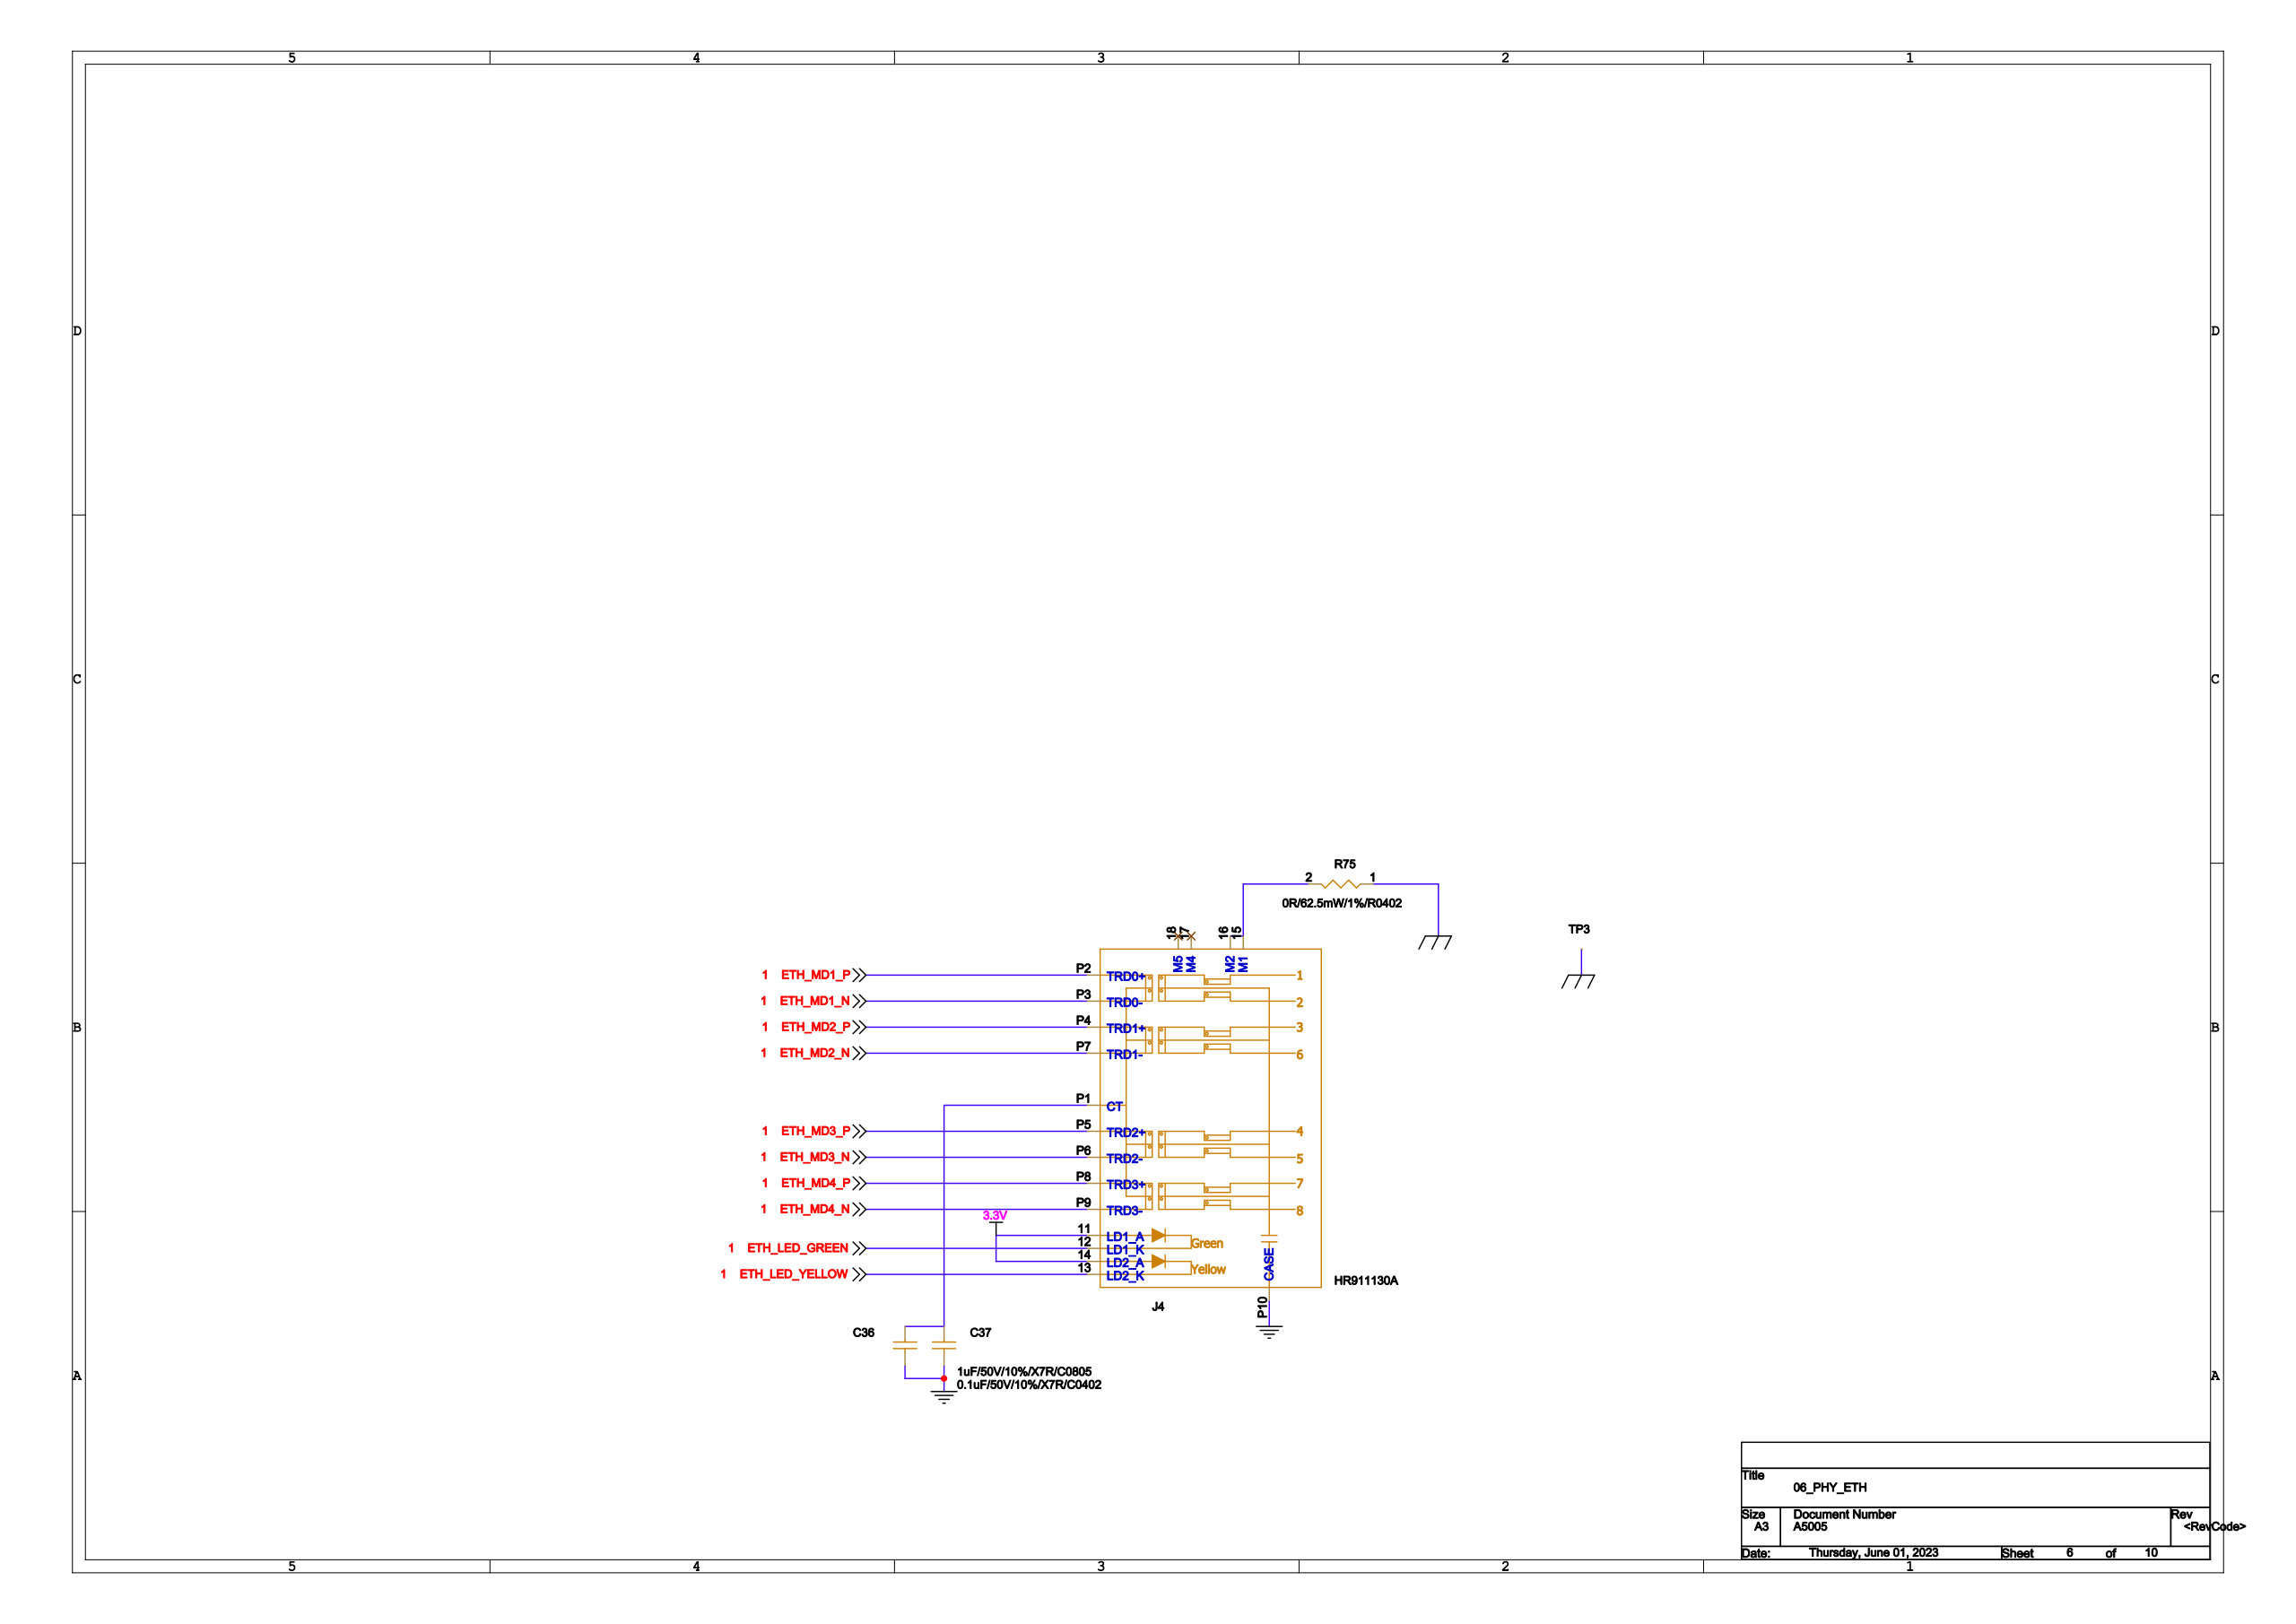Circuit board | Cadence Allegro | 480 parts | 625 nets | one sheet of the schematic
Parts on this sheet (reference | value | footprint):
C36 | 1uF/50V/10%/X7R/C0805 | 0805
C37 | 0.1uF/50V/10%/X7R/C0402 | 0402
R75 | 0R/62.5mW/1%/R0402 | 0402
TP3 | TEST POINT A | HOLE2-3_5
Nets of these parts (net: part-pin ...):
AGND: C36-2 C37-2
GND_EARTH: R75-1 TP3-1
N23857542: C36-1 C37-1
N23857284: R75-2